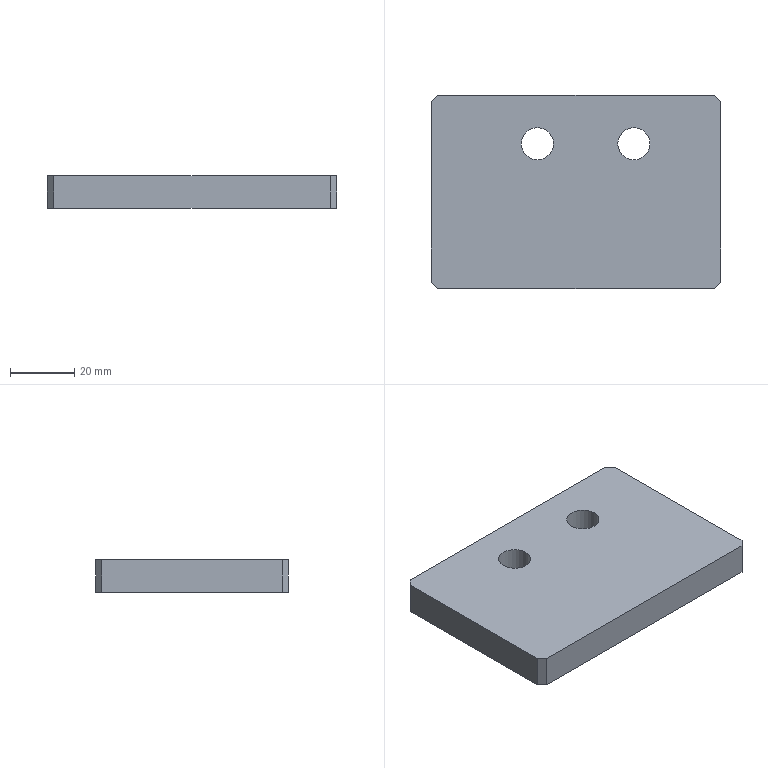NC program | NX | posted with a generic post | part box 90 x 60 x 10 mm
Lines 540 to 1827 of 1827:
(ADAPTIVE_MILLING_COPY , TOOL : D12开粗)
N1036 T02 M6
N1038 G54
N1040 G17 G0 G90 X-59.569 Y-30.89 S3000 M3
N1042 G43 Z20. H2
N1044 Z3.1
N1046 G94 G1 X-59.419 Y-30.888 Z2.163 F1500.
N1048 X-59.269 Y-30.885 Z1.792
N1050 X-59.119 Y-30.883 Z1.52
N1052 X-58.969 Y-30.88 Z1.3
N1054 X-58.819 Y-30.878 Z1.116
N1056 X-58.669 Y-30.875 Z0.958
N1058 X-58.519 Y-30.873 Z0.82
N1060 X-58.369 Y-30.87 Z0.7
N1062 X-58.219 Y-30.867 Z0.595
N1064 X-58.069 Y-30.865 Z0.502
N1066 X-57.919 Y-30.862 Z0.421
N1068 X-57.769 Y-30.86 Z0.35
N1070 X-57.619 Y-30.857 Z0.29
N1072 X-57.469 Y-30.855 Z0.238
N1074 X-57.319 Y-30.852 Z0.195
N1076 X-57.169 Y-30.85 Z0.161
N1078 X-57.019 Y-30.847 Z0.134
N1080 X-56.869 Y-30.845 Z0.115
N1082 X-56.719 Y-30.842 Z0.104
N1084 X-56.569 Y-30.84 Z0.1
N1086 X-54.659 Y-30.808
N1088 G3 X-53.548 Y-30.03 R1.212
N1090 X-53.17 Y-27.731 R8.892
N1092 X-53.004 Y-19.97 R127.75
N1094 G1 X-52.999 Y-14.169
N1096 X-52.997 Y32.519
N1098 G2 X-50.378 Y37.762 R6.759
N1100 X-45.571 Y39.899 R11.024
N1102 X-39.916 Y40.431 R33.002
N1104 X-28.979 Y40.499 R545.05
N1106 G1 X45.014 Y40.497
N1108 G2 X50.26 Y37.882 R6.758
N1110 X52.398 Y33.076 R11.015
N1112 X52.936 Y27.233 R33.716
N1114 X52.998 Y16.484 R602.889
N1116 G1 X52.997 Y-32.512
N1118 G2 X50.383 Y-37.757 R6.757
N1120 X45.576 Y-39.897 R11.021
N1122 X39.734 Y-40.436 R33.627
N1124 X28.984 Y-40.499 R598.92
N1126 G1 X-45.011 Y-40.497
N1128 G2 X-50.217 Y-37.931 R6.744
N1130 X-52.518 Y-31.955 R10.821
N1132 X-52.587 Y-26.958 R47.485
N1134 G3 X-52.499 Y-14.793 R707.62
N1136 G1 X-52.497 Y30.394
N1138 G2 X-48.711 Y37.306 R8.485
N1140 X-43.265 Y39.414 R13.689
N1142 X-36.542 Y39.944 R43.936
N1144 X-25.855 Y39.998 R696.998
N1146 G1 X42.893 Y39.997
N1148 G2 X49.808 Y36.209 R8.485
N1150 X51.913 Y30.767 R13.682
N1152 X52.446 Y23.92 R44.535
N1154 X52.498 Y12.92 R714.019
N1156 G1 X52.496 Y-30.39
N1158 G2 X48.799 Y-37.243 R8.475
N1160 X43.429 Y-39.382 R13.467
N1162 X37.022 Y-39.932 R40.74
N1164 X25.522 Y-39.998 R644.298
N1166 G1 X-42.89 Y-39.997
N1168 G2 X-50.102 Y-35.708 R8.457
N1170 X-51.749 Y-30.501 R13.432
N1172 X-52.014 Y-24.698 R49.366
N1174 G1 X-51.999 Y-15.168
N1176 X-51.998 Y28.27
N1178 G2 X-47.019 Y37.045 R9.749
N1180 X-41.174 Y38.973 R16.302
N1182 X-33.945 Y39.451 R55.428
N1184 X-24.32 Y39.498 R682.976
N1186 G1 X40.792 Y39.497
N1188 G2 X49.543 Y34.524 R9.746
N1190 X51.462 Y28.74 R16.226
N1192 X51.953 Y21.325 R55.538
N1194 X51.997 Y10.762 R717.555
N1196 G1 X51.996 Y-28.288
N1198 G2 X47.025 Y-37.04 R9.747
N1200 X41.178 Y-38.971 R16.292
N1202 X33.637 Y-39.456 R57.142
N1204 X23.324 Y-39.498 R714.456
N1206 G1 X-40.765 Y-39.497
N1208 G2 X-46.89 Y-37.527 R9.612
N1210 X-50.43 Y-32.205 R10.902
N1212 X-51.379 Y-26.298 R23.347
N1214 X-51.5 Y-18.487 R163.612
N1216 G1 X-51.498 Y26.444
N1218 G2 X-50.572 Y31.508 R12.25
N1220 X-45.244 Y36.861 R10.95
N1222 X-39.06 Y38.556 R19.433
N1224 X-31.012 Y38.967 R74.188
N1226 G1 X-21.199 Y38.997
N1228 X38.956 Y38.996
N1230 G2 X44.075 Y38.04 R12.18
N1232 X49.414 Y32.633 R10.992
N1234 X51.055 Y26.564 R19.568
N1236 X51.465 Y18.641 R73.264
N1238 G1 X51.497 Y8.829
N1240 X51.496 Y-26.453
N1242 G2 X50.54 Y-31.573 R12.182
N1244 X45.238 Y-36.861 R10.959
N1246 X39.116 Y-38.548 R19.361
N1248 X30.943 Y-38.967 R74.081
N1250 G1 X21.131 Y-38.998
N1252 X-38.953 Y-38.996
N1254 G2 X-43.781 Y-38.15 R12.071
N1256 X-49.101 Y-32.875 R10.495
N1258 X-50.645 Y-27.041 R18.389
N1260 X-50.984 Y-19.239 R74.744
N1262 G1 X-50.999 Y-11.614
N1264 X-50.998 Y24.811
N1266 G2 X-50.358 Y29.622 R15.163
N1268 X-44.803 Y36.031 R11.276
N1270 X-38.427 Y37.958 R19.18
N1272 X-30.26 Y38.454 R66.913
N1274 X-19.698 Y38.497 R723.605
N1276 G1 X37.331 Y38.496
N1278 G2 X42.141 Y37.851 R15.119
N1280 X48.569 Y32.23 R11.299
N1282 X50.442 Y26.038 R19.12
N1284 X50.948 Y18.06 R64.164
N1286 X50.997 Y6.748 R739.344
N1288 G1 X50.995 Y-24.828
N1290 G2 X50.331 Y-29.698 R15.054
N1292 X44.729 Y-36.069 R11.307
N1294 X38.472 Y-37.951 R19.238
N1296 X30.305 Y-38.453 R66.231
N1298 X19.993 Y-38.497 R712.26
N1300 G1 X-37.328 Y-38.496
N1302 G2 X-42.015 Y-37.872 R14.739
N1304 X-48.266 Y-32.372 R10.913
N1306 X-50.058 Y-26.153 R18.659
N1308 X-50.464 Y-18.856 R65.496
N1310 X-50.499 Y-8.919 R714.694
N1312 G1 Y22.955
N1314 G2 X-50.093 Y27.677 R20.632
N1316 X-44.089 Y35.381 R11.711
N1318 X-37.741 Y37.378 R19.475
N1320 X-29.766 Y37.935 R61.44
N1322 X-17.704 Y37.997 R739.177
N1324 G1 X35.581 Y37.996
N1326 G2 X40.359 Y37.548 R19.649
N1328 X47.878 Y31.593 R11.713
N1330 X49.877 Y25.245 R19.451
N1332 X50.432 Y17.396 R60.715
N1334 X50.496 Y4.959 R746.772
N1336 G1 Y-23.078
N1338 G2 X50.048 Y-27.857 R19.657
N1340 X44.094 Y-35.376 R11.714
N1342 X37.561 Y-37.405 R19.666
N1344 X29.334 Y-37.944 R65.096
N1346 X17.397 Y-37.997 R755.241
N1348 G1 X-35.716 Y-37.996
N1350 G2 X-40.426 Y-37.51 R18.131
N1352 X-47.589 Y-31.648 R11.386
N1354 X-49.483 Y-25.329 R19.143
N1356 X-49.957 Y-17.473 R65.04
N1358 X-49.999 Y-7.161 R715.418
N1360 G1 X-49.998 Y21.58
N1362 G2 X-49.606 Y26.555 R23.599
N1364 X-43.258 Y34.825 R12.177
N1366 X-36.784 Y36.851 R20.187
N1368 X-28.498 Y37.433 R63.335
N1370 X-16.498 Y37.496 R737.911
N1372 G1 X34.081
N1374 G2 X39.055 Y37.104 R23.631
N1376 X47.327 Y30.753 R12.176
N1378 X49.38 Y24.095 R20.39
N1380 X49.94 Y15.619 R66.815
N1382 X49.996 Y4.619 R715.925
N1384 G1 X49.995 Y-21.64
N1386 G2 X49.604 Y-26.553 R23.37
N1388 X43.254 Y-34.825 R12.176
N1390 X36.759 Y-36.854 R20.234
N1392 X28.598 Y-37.431 R62.902
N1394 X15.911 Y-37.497 R756.324
N1396 G1 X-33.953 Y-37.496
N1398 G2 X-38.744 Y-37.149 R24.037
N1400 X-46.94 Y-30.942 R11.836
N1402 X-48.929 Y-24.45 R19.689
N1404 X-49.45 Y-16.285 R65.25
N1406 X-49.498 Y-4.973 R739.456
N1408 G1 X-49.497 Y20.205
N1410 G2 X-49.14 Y25.372 R27.452
N1412 X-42.409 Y34.302 R12.608
N1414 X-35.615 Y36.366 R21.2
N1416 X-27.015 Y36.937 R68.595
N1418 X-14.64 Y36.996 R759.565
N1420 G1 X32.706 Y36.995
N1422 G2 X37.873 Y36.638 R27.447
N1424 X46.761 Y29.985 R12.59
N1426 X48.823 Y23.395 R20.784
N1428 X49.422 Y15.173 R63.113
N1430 X49.496 Y2.111 R755.001
N1432 G1 X49.495 Y-20.203
N1434 G2 X49.138 Y-25.37 R27.447
N1436 X42.431 Y-34.288 R12.598
N1438 X35.769 Y-36.341 R20.997
N1440 X27.358 Y-36.93 R65.469
N1442 X14.609 Y-36.996 R758.776
N1444 G1 X-32.64
N1446 G2 X-37.683 Y-36.651 R26.828
N1448 X-46.442 Y-30.007 R12.311
N1450 X-48.398 Y-23.508 R20.608
N1452 X-48.942 Y-15.282 R65.734
N1454 X-48.998 Y-3.282 R748.174
N1456 G1 X-48.997 Y18.956
N1458 G2 X-48.654 Y24.312 R30.683
N1460 X-41.645 Y33.754 R12.991
N1462 X-34.923 Y35.817 R21.6
N1464 X-26.388 Y36.424 R66.253
N1466 X-13.326 Y36.496 R760.292
N1468 G1 X31.456 Y36.495
N1470 G2 X36.813 Y36.152 R30.68
N1472 X46.257 Y29.139 R12.991
N1474 X48.327 Y22.351 R21.706
N1476 X48.928 Y13.69 R67.775
N1478 X48.995 Y1.003 R755.917
N1480 G1 X48.994 Y-19.016
N1482 G2 X48.652 Y-24.31 R30.377
N1484 X41.639 Y-33.755 R12.989
N1486 X34.852 Y-35.826 R21.702
N1488 X26.255 Y-36.427 R67.324
N1490 X13.192 Y-36.496 R761.577
N1492 G1 X-31.453 Y-36.495
N1494 G2 X-36.623 Y-36.161 R29.577
N1496 X-45.833 Y-29.326 R12.696
N1498 X-47.872 Y-22.599 R21.178
N1500 X-48.44 Y-14.061 R67.815
N1502 X-48.497 Y-2.061 R748.385
N1504 G1 X-48.496 Y17.768
N1506 G2 X-48.163 Y23.313 R33.923
N1508 X-40.875 Y33.225 R13.35
N1510 X-33.967 Y35.314 R22.312
N1512 X-25.306 Y35.923 R68.534
N1514 X-11.932 Y35.995 R770.057
N1516 G1 X30.368 Y35.994
N1518 G2 X35.913 Y35.644 R32.71
N1520 X45.724 Y28.375 R13.34
N1522 X47.814 Y21.465 R22.311
N1524 X48.421 Y12.868 R68.251
N1526 X48.495 Y0.868 R720.862
N1528 G1 X48.493 Y-17.869
N1530 G2 X48.143 Y-23.414 R32.688
N1532 X40.876 Y-33.222 R13.341
N1534 X34.028 Y-35.303 R22.252
N1536 X25.431 Y-35.92 R67.417
N1538 X11.994 Y-35.995 R766.793
N1540 G1 X-30.306 Y-35.994
N1542 G2 X-35.725 Y-35.649 R31.627
N1544 X-45.278 Y-28.579 R13.059
N1546 X-47.349 Y-21.726 R21.763
N1548 X-47.936 Y-13.002 R69.124
N1550 X-47.997 Y-0.628 R755.649
N1552 G1 X-47.995 Y16.768
N1554 G2 X-47.646 Y22.5 R35.2
N1556 X-40.091 Y32.716 R13.677
N1558 X-33.167 Y34.793 R22.909
N1560 X-24.32 Y35.42 R69.666
N1562 X-10.571 Y35.495 R775.803
N1564 G1 X29.081 Y35.494
N1566 G2 X34.816 Y35.174 R37.476
N1568 X45.214 Y27.595 R13.684
N1570 X47.292 Y20.671 R22.893
N1572 X47.917 Y11.949 R69.041
N1574 X47.994 Y-0.426 R727.241
N1576 G1 X47.993 Y-16.578
N1578 G2 X47.674 Y-22.313 R37.496
N1580 X40.088 Y-32.716 R13.688
N1582 X33.17 Y-34.791 R22.924
N1584 X24.449 Y-35.417 R68.877
N1586 X10.699 Y-35.495 R772.946
N1588 G1 X-29.015 Y-35.494
N1590 G2 X-34.563 Y-35.187 R36.616
N1592 X-44.84 Y-27.629 R13.457
N1594 X-46.857 Y-20.695 R22.84
N1596 X-47.434 Y-11.907 R72.379
N1598 X-47.497 Y0.717 R763.165
N1600 G1 X-47.495 Y15.518
N1602 G2 X-47.192 Y21.317 R40.767
N1604 X-43.007 Y29.661 R14.033
N1606 X-36.223 Y33.426 R16.757
N1608 X-28.467 Y34.699 R35.764
N1610 X-17.473 Y34.984 R174.966
N1612 G1 X-9.91 Y34.995
N1614 X27.893 Y34.994
N1616 G2 X33.817 Y34.69 R41.623
N1618 X42.07 Y30.6 R14.047
N1620 X45.925 Y23.728 R16.697
N1622 X47.203 Y15.909 R35.882
N1624 X47.483 Y5.102 R175.284
N1626 G1 X47.494 Y-3.148
N1628 X47.493 Y-15.391
N1630 G2 X47.19 Y-21.315 R41.672
N1632 X43.102 Y-29.567 R14.047
N1634 X36.466 Y-33.35 R16.55
N1636 X28.783 Y-34.675 R34.459
N1638 X17.602 Y-34.983 R165.961
N1640 G1 X9.352 Y-34.995
N1642 X-27.828 Y-34.994
N1644 G2 X-33.565 Y-34.7 R40.526
N1646 X-42.02 Y-30.309 R13.761
N1648 X-45.559 Y-23.6 R16.821
N1650 X-46.723 Y-16.14 R36.323
N1652 X-46.991 Y-4.082 R198.021
N1654 G1 X-46.996 Y2.105
N1656 X-46.995 Y14.33
N1658 G2 X-46.71 Y20.319 R45.501
N1660 X-43.484 Y27.928 R14.662
N1662 X-36.738 Y32.487 R15.777
N1664 X-29.233 Y34.056 R30.463
N1666 X-18.932 Y34.467 R120.399
N1668 G1 X-9.307 Y34.494
N1670 X26.831 Y34.493
N1672 G2 X32.819 Y34.208 R45.449
N1674 X40.428 Y30.98 R14.652
N1676 X44.955 Y24.323 R15.724
N1678 X46.547 Y16.82 R30.062
N1680 X46.967 Y6.456 R119.196
N1682 G1 X46.994 Y-3.168
N1684 G2 X46.958 Y-17.015 R894.236
N1686 X46.166 Y-22.883 R22.934
N1688 X38.883 Y-31.545 R14.131
N1690 X31.739 Y-33.737 R23.419
N1692 X22.77 Y-34.407 R69.21
N1694 X8.708 Y-34.494 R725.36
N1696 G1 X-26.703 Y-34.493
N1698 G2 X-32.752 Y-34.189 R42.972
N1700 X-40.769 Y-30.384 R14.184
N1702 X-44.818 Y-23.562 R16.298
N1704 X-46.175 Y-15.822 R34.003
N1706 X-46.484 Y-4.829 R161.702
N1708 G1 X-46.496 Y3.421
N1710 G2 X-46.454 Y16.267 R676.278
N1712 X-45.584 Y22.374 R22.998
N1714 X-38.26 Y30.986 R14.365
N1716 X-30.939 Y33.231 R23.843
N1718 X-21.72 Y33.909 R71.389
N1720 X-7.283 Y33.994 R768.457
N1722 G1 X25.643 Y33.993
N1724 G2 X32.007 Y33.702 R49.117
N1726 X39.552 Y30.628 R15.084
N1728 X44.364 Y23.794 R15.81
N1730 X46.022 Y16.18 R30.054
N1732 X46.463 Y5.818 R115.982
N1734 G1 X46.493 Y-3.807
N1736 G2 X46.451 Y-16.265 R648.348
N1738 X45.582 Y-22.372 R22.999
N1740 X38.265 Y-30.981 R14.361
N1742 X31.185 Y-33.19 R23.535
N1744 X22.095 Y-33.899 R67.862
N1746 X7.283 Y-33.994 R698.792
N1748 G1 X-25.578 Y-33.993
N1750 G2 X-31.754 Y-33.707 R47.373
N1752 X-39.296 Y-30.574 R14.789
N1754 X-43.946 Y-23.834 R15.682
N1756 X-45.535 Y-16.46 R29.732
N1758 X-45.967 Y-6.16 R115.012
N1760 G1 X-45.996 Y4.153
N1762 G2 X-45.941 Y15.704 R452.456
N1764 X-45.004 Y21.863 R22.721
N1766 X-37.557 Y30.474 R14.601
N1768 X-30.234 Y32.712 R24.223
N1770 X-21.016 Y33.402 R71.367
N1772 X-7.267 Y33.493 R695.731
N1774 G1 X24.518
N1776 G2 X31.008 Y33.224 R54.432
N1778 X38.224 Y30.603 R15.779
N1780 X43.579 Y23.756 R15.519
N1782 X45.418 Y16.253 R28.081
N1784 X45.942 Y6.459 R95.891
N1786 X45.993 Y-5.229 R761.677
N1788 X45.938 Y-15.702 R398.582
N1790 X45.002 Y-21.862 R22.729
N1792 X37.562 Y-30.469 R14.6
N1794 X30.239 Y-32.71 R24.23
N1796 X21.021 Y-33.402 R71.255
N1798 X7.272 Y-33.494 R689.902
N1800 G1 X-24.453 Y-33.493
N1802 G2 X-30.755 Y-33.227 R52.481
N1804 X-38.002 Y-30.53 R15.452
N1806 X-43.165 Y-23.783 R15.41
N1808 X-44.952 Y-16.331 R28.096
N1810 X-45.455 Y-6.223 R100.534
N1812 X-45.495 Y5.527 R787.676
N1814 X-45.422 Y15.263 R274.803
N1816 X-44.387 Y21.468 R22.131
N1818 X-36.847 Y29.973 R14.832
N1820 X-29.458 Y32.207 R24.724
N1822 X-20.615 Y32.889 R70.497
N1824 X-6.554 Y32.993 R617.429
N1826 G1 X23.496 Y32.992
N1828 G2 X30.175 Y32.725 R57.816
N1830 X37.319 Y30.25 R16.264
N1832 X42.997 Y23.22 R15.591
N1834 X44.889 Y15.664 R28.061
N1836 X45.436 Y5.872 R93.584
N1838 X45.452 Y-14.365 R851.165
N1840 X44.651 Y-20.61 R25.74
N1842 X36.94 Y-29.922 R14.805
N1844 X29.563 Y-32.188 R24.482
N1846 X20.347 Y-32.895 R70.992
N1848 X5.222 Y-32.993 R705.308
N1850 G1 X-23.328
N1852 G2 X-29.757 Y-32.747 R58.397
N1854 X-36.853 Y-30.339 R16.169
N1856 X-42.475 Y-23.489 R15.342
N1858 X-44.388 Y-16.004 R27.328
N1860 X-44.938 Y-6.337 R90.537
N1862 X-44.955 Y13.462 R849.616
N1864 X-44.195 Y19.714 R27.14
N1866 X-36.224 Y29.433 R15.024
N1868 X-28.84 Y31.68 R24.95
N1870 X-19.873 Y32.384 R70.359
N1872 X-5.124 Y32.493 R628.055
N1874 G1 X22.364 Y32.492
N1876 G2 X29.23 Y32.242 R63.749
N1878 X36.313 Y29.956 R16.939
N1880 X42.282 Y22.995 R15.551
N1882 X44.29 Y15.602 R26.857
N1884 X44.918 Y5.941 R83.161
N1886 X44.953 Y-13.434 R753.505
N1888 X44.216 Y-19.626 R27.436
N1890 X36.229 Y-29.428 R15.023
N1892 X28.905 Y-31.667 R24.864
N1894 X19.565 Y-32.392 R71.306
N1896 X5.565 Y-32.493 R648.052
N1898 G1 X-22.297 Y-32.492
N1900 G2 X-29.038 Y-32.235 R60.414
N1902 X-36.095 Y-29.882 R16.519
N1904 X-41.891 Y-22.954 R15.463
N1906 X-43.841 Y-15.54 R27.151
N1908 X-44.421 Y-6.313 R84.039
N1910 X-44.454 Y12.624 R716.587
N1912 X-43.689 Y19.001 R27.965
N1914 X-35.694 Y28.851 R15.184
N1916 X-28.318 Y31.139 R24.924
N1918 X-18.917 Y31.886 R70.795
N1920 X-4.168 Y31.992 R650.065
N1922 G1 X21.382
N1924 G2 X28.499 Y31.735 R66.483
N1926 X35.592 Y29.484 R17.303
N1928 X41.782 Y22.296 R15.734
N1930 X43.805 Y14.709 R27.55
N1932 X44.415 Y5.172 R85.471
N1934 X44.443 Y-12.89 R576.077
N1936 X43.634 Y-19.198 R26.829
N1938 X35.654 Y-28.869 R15.193
N1940 X28.395 Y-31.124 R24.881
N1942 X19.183 Y-31.878 R68.93
N1944 X4.372 Y-31.992 R603.076
N1946 G1 X-21.241
N1948 G2 X-28.108 Y-31.75 R66.124
N1950 X-35.101 Y-29.572 R17.199
N1952 X-41.277 Y-22.496 R15.514
N1954 X-43.316 Y-14.918 R27.092
N1956 X-43.917 Y-5.567 R83.745
N1958 X-43.941 Y12.182 R531.225
N1960 X-43.133 Y18.491 R27.342
N1962 X-34.96 Y28.379 R15.385
N1964 X-27.391 Y30.667 R25.652
N1966 X-18.113 Y31.384 R73.258
N1968 X-3.676 Y31.492 R634.739
N1970 G1 X20.436 Y31.491
N1972 G2 X27.554 Y31.253 R72.029
N1974 X34.58 Y29.182 R18.034
N1976 X41.11 Y21.983 R15.725
N1978 X43.255 Y14.301 R27.03
N1980 X43.899 Y5.017 R80.432
N1982 X43.939 Y-12.17 R476.093
N1984 X43.101 Y-18.6 R27.123
N1986 X35.048 Y-28.331 R15.368
N1988 X27.481 Y-30.65 R25.445
N1990 X18.142 Y-31.383 R72.387
N1992 X3.705 Y-31.492 R624.013
N1994 G1 X-20.283
N1996 G2 X-27.338 Y-31.247 R68.888
N1998 X-34.344 Y-29.119 R17.608
N2000 X-40.673 Y-22.025 R15.612
N2002 X-42.762 Y-14.52 R26.795
N2004 X-43.416 Y-4.736 R82.159
N2006 X-43.431 Y11.638 R423.949
N2008 X-42.52 Y18.183 R26.615
N2010 X-34.485 Y27.778 R15.517
N2012 X-26.992 Y30.11 R25.374
N2014 X-17.592 Y30.875 R70.853
N2016 X-1.718 Y30.992 R642.346
N2018 G1 X19.394 Y30.991
N2020 G2 X26.7 Y30.762 R77.721
N2022 X33.645 Y28.828 R18.692
N2024 X40.553 Y21.428 R15.817
N2026 X42.688 Y14.001 R26.751
N2028 X43.386 Y4.658 R76.209
N2030 X43.427 Y-11.653 R377.553
N2032 X42.548 Y-18.077 R26.764
N2034 X34.433 Y-27.802 R15.525
N2036 X26.811 Y-30.137 R25.703
N2038 X17.41 Y-30.88 R72.888
N2040 X2.598 Y-30.992 R628.724
N2042 G1 X-19.202 Y-30.991
N2044 G2 X-26.445 Y-30.76 R75.302
N2046 X-33.317 Y-28.816 R18.354
N2048 X-40.105 Y-21.484 R15.693
N2050 X-42.226 Y-13.994 R26.769
N2052 X-42.902 Y-4.461 R78.861
N2054 X-42.931 Y10.788 R372.385
N2056 X-42.079 Y17.279 R27.95
N2058 X-33.849 Y27.265 R15.69
N2060 X-26.231 Y29.615 R25.836
N2062 X-16.768 Y30.375 R72.478
N2064 X-0.644 Y30.491 R659.501
N2066 G1 X18.469
N2068 G2 X26.087 Y30.247 R78.624
N2070 X33.081 Y28.278 R18.867
N2072 X40.029 Y20.81 R15.986
N2074 X42.206 Y13.139 R27.259
N2076 X42.899 Y3.295 R81.438
N2078 X42.912 Y-11.203 R300.444
N2080 X41.943 Y-17.739 R25.936
N2082 X33.873 Y-27.25 R15.671
N2084 X26.315 Y-29.598 R25.708
N2086 X16.791 Y-30.374 R71.856
N2088 X0.605 Y-30.492 R657.571
N2090 G1 X-18.258 Y-30.491
N2092 G2 X-25.751 Y-30.252 R77.544
N2094 X-32.685 Y-28.299 R18.637
N2096 X-39.548 Y-20.929 R15.832
N2098 X-41.697 Y-13.441 R26.817
N2100 X-42.395 Y-3.91 R77.606
N2102 X-42.41 Y10.526 R282.113
N2104 X-41.425 Y17.122 R26.283
N2106 X-33.161 Y26.782 R15.842
N2108 X-25.472 Y29.121 R26.31
N2110 X-16.196 Y29.867 R72.956
N2112 X-0.759 Y29.991 R604.001
N2114 G1 X18.228 Y29.989
N2116 G2 X25.657 Y29.714 R71.025
N2118 X32.744 Y27.609 R18.72
N2120 X39.519 Y20.172 R16.182
N2122 X41.675 Y12.617 R27.376
N2124 X42.387 Y2.962 R78.943
N2126 X42.4 Y-10.662 R247.08
N2128 X41.364 Y-17.311 R25.587
N2130 X33.234 Y-26.742 R15.823
N2132 X25.551 Y-29.105 R26.114
N2134 X16.151 Y-29.868 R72.626
N2136 X-0.598 Y-29.991 R659.571
N2138 G1 X-18.086 Y-29.989
N2140 G2 X-25.265 Y-29.724 R69.895
N2142 X-32.352 Y-27.623 R18.514
N2144 X-39.025 Y-20.31 R16.022
N2146 X-41.216 Y-12.573 R27.344
N2148 X-41.897 Y-2.978 R80.637
N2150 X-41.907 Y9.77 R242.832
N2152 X-40.912 Y16.49 R26.77
N2154 X-32.66 Y26.208 R15.965
N2156 X-24.853 Y28.605 R26.385
N2158 X-15.453 Y29.366 R73.385
N2160 X-0.079 Y29.49 R599.195
N2162 G1 X17.284 Y29.489
N2164 G2 X24.714 Y29.237 R77.294
N2166 X31.725 Y27.309 R19.514
N2168 X38.898 Y19.773 R16.197
N2170 X41.172 Y11.925 R27.418
N2172 X41.881 Y2.394 R79.068
N2174 X41.897 Y-9.916 R214.326
N2176 X40.884 Y-16.571 R26.237
N2178 X32.666 Y-26.201 R15.961
N2180 X25.05 Y-28.57 R26.149
N2182 X15.59 Y-29.361 R71.472
N2184 X-1.221 Y-29.491 R631.424
N2186 G1 X-17.084 Y-29.489
N2188 G2 X-24.451 Y-29.233 R74.928
N2190 X-31.448 Y-27.261 R19.132
N2192 X-38.444 Y-19.822 R16.086
N2194 X-40.677 Y-12.102 R27.22
N2196 X-41.396 Y-2.197 R80.139
N2198 X-41.377 Y9.614 R184.313
N2200 X-40.256 Y16.312 R25.227
N2202 X-32.19 Y25.62 R16.061
N2204 X-24.345 Y28.073 R26.293
N2206 X-14.822 Y28.861 R72.746
N2208 X1.052 Y28.99 R601.271
N2210 G1 X16.415 Y28.989
N2212 G2 X24.094 Y28.726 R78.463
N2214 X31.163 Y26.769 R19.682
N2216 X38.339 Y19.252 R16.301
N2218 X40.612 Y11.603 R27.131
N2220 X41.364 Y2.202 R74.823
N2222 X41.369 Y-9.671 R170.277
N2224 X40.215 Y-16.426 R24.907
N2226 X32.048 Y-25.689 R16.091
N2228 X24.253 Y-28.086 R26.596
N2230 X14.729 Y-28.863 R73.64
N2232 X-1.77 Y-28.99 R633.569
N2234 G1 X-16.195 Y-28.989
N2236 G2 X-23.688 Y-28.736 R78.263
N2238 X-30.76 Y-26.785 R19.547
N2240 X-37.895 Y-19.273 R16.203
N2242 X-40.123 Y-11.734 R27.06
N2244 X-40.881 Y-1.958 R76.323
N2246 X-40.858 Y9.165 R153.521
N2248 X-39.648 Y15.974 R24.611
N2250 X-31.55 Y25.123 R16.195
N2252 X-23.88 Y27.535 R26.387
N2254 X-14.485 Y28.347 R70.631
N2256 X3.076 Y28.49 R612.418
N2258 G1 X15.564 Y28.488
N2260 G2 X23.369 Y28.227 R81.493
N2262 X30.451 Y26.31 R20.127
N2264 X37.811 Y18.672 R16.41
N2266 X40.122 Y10.842 R27.499
N2268 X40.867 Y1.315 R77.049
N2270 X40.844 Y-9.307 R137.405
N2272 X39.576 Y-16.166 R24.043
N2274 X31.564 Y-25.113 R16.188
N2276 X23.897 Y-27.53 R26.352
N2278 X14.19 Y-28.356 R71.737
N2280 X-3.059 Y-28.49 R637.467
N2282 G1 X-15.359 Y-28.489
N2284 G2 X-23.164 Y-28.216 R77.999
N2286 X-30.168 Y-26.261 R19.64
N2288 X-37.355 Y-18.711 R16.321
N2290 X-39.617 Y-11.067 R27.252
N2292 X-40.372 Y-1.478 R75.896
N2294 X-40.338 Y8.707 R128.277
N2296 X-39.084 Y15.506 R24.307
N2298 X-30.834 Y24.667 R16.35
N2300 X-23.096 Y27.052 R26.895
N2302 X-13.512 Y27.854 R73.287
N2304 X2.299 Y27.989 R579.941
N2306 G1 X13.974
N2308 G2 X22.157 Y27.775 R101.775
N2310 X29.121 Y26.14 R21.677
N2312 X37.237 Y18.192 R16.437
N2314 X39.567 Y10.501 R27.207
N2316 X40.358 Y0.852 R74.548
N2318 X40.298 Y-9.206 R109.209
N2320 X38.835 Y-16.149 R22.673
N2322 X30.749 Y-24.707 R16.385
N2324 X22.94 Y-27.075 R27.229
N2326 X13.292 Y-27.86 R75.193
N2328 X-3.582 Y-27.99 R647.562
N2330 X-18.757 Y-27.94 R864.103
N2332 X-25.64 Y-27.181 R33.424
N2334 X-36.725 Y-18.34 R16.299
N2336 X-39.082 Y-10.589 R26.983
N2338 X-39.862 Y-1.003 R74.177
N2340 X-39.799 Y8.494 R104.034
N2342 X-38.389 Y15.386 R23.175
N2344 X-30.355 Y24.094 R16.44
N2346 X-22.504 Y26.537 R26.921
N2348 X-12.67 Y27.357 R74.351
N2350 X4.204 Y27.489 R637.079
N2352 X18.566 Y27.432 R696.859
N2354 X25.386 Y26.67 R33.837
N2356 X36.665 Y17.712 R16.53
N2358 X39.043 Y9.968 R27.179
N2360 X39.852 Y0.259 R73.698
N2362 X39.754 Y-8.986 R88.643
N2364 X38.147 Y-15.961 R21.814
N2366 X30.213 Y-24.162 R16.498
N2368 X22.53 Y-26.531 R27.116
N2370 X12.947 Y-27.348 R72.791
N2372 X-4.302 Y-27.489 R612.109
N2374 X-18.164 Y-27.436 R705.169
N2376 X-24.925 Y-26.694 R33.811
N2378 X-36.15 Y-17.858 R16.408
N2380 X-38.566 Y-10. R27.009
N2382 X-39.362 Y-0.165 R74.573
N2384 X-39.212 Y8.766 R78.147
N2386 X-37.433 Y15.821 R21.127
N2388 X-29.722 Y23.601 R16.62
N2390 X-21.804 Y26.042 R27.289
N2392 X-11.97 Y26.855 R75.298
N2394 X5.591 Y26.989 R665.399
N2396 X18.141 Y26.922 R475.392
N2398 X25.016 Y26.101 R32.712
N2400 X36.103 Y17.217 R16.616
N2402 X38.532 Y9.36 R27.251
N2404 X39.358 Y-0.849 R74.986
N2406 X39.151 Y-9.278 R65.815
N2408 X37.028 Y-16.617 R19.872
N2410 X29.337 Y-23.788 R16.798
N2412 X21.385 Y-26.107 R28.319
N2414 X11.545 Y-26.867 R79.925
N2416 X-5.641 Y-26.989 R710.751
N2418 X-17.941 Y-26.919 R462.341
N2420 X-24.75 Y-26.076 R31.722
N2422 X-35.662 Y-17.211 R16.52
N2424 X-38.062 Y-9.343 R27.327
N2426 X-38.867 Y1.055 R75.86
N2428 X-38.6 Y9.044 R58.071
N2430 X-36.222 Y16.561 R19.338
N2432 X-28.623 Y23.337 R17.032
N2434 X-20.717 Y25.61 R28.757
N2436 X-10.565 Y26.374 R82.211
N2438 X6.185 Y26.488 R740.157
N2440 X17.921 Y26.403 R365.762
N2442 X24.905 Y25.462 R30.659
N2444 X35.617 Y16.575 R16.714
N2446 X38.019 Y8.775 R27.456
N2448 X38.855 Y-1.934 R74.521
N2450 X38.508 Y-9.668 R49.416
N2452 X35.646 Y-17.467 R18.35
N2454 X28.058 Y-23.591 R17.411
N2456 X19.917 Y-25.724 R30.66
N2458 X9.882 Y-26.391 R91.673
N2460 X-6.18 Y-26.489 R827.798
N2462 X-17.604 Y-26.404 R342.957
N2464 X-24.464 Y-25.48 R30.352
N2466 X-35.101 Y-16.715 R16.6
N2468 X-37.531 Y-8.859 R27.27
N2470 X-38.356 Y2.162 R73.988
N2472 X-37.899 Y9.701 R43.079
N2474 X-34.363 Y17.939 R17.684
N2476 X-26.789 Y23.366 R18.106
N2478 X-18.538 Y25.317 R33.062
N2480 X-7.685 Y25.92 R107.817
N2482 X16.177 Y25.937 R979.786
N2484 X23.132 Y25.241 R37.672
N2486 X32.415 Y19.992 R16.931
N2488 X36.536 Y12.375 R20.185
N2490 X38.057 Y3.647 R41.409
N2492 X38.184 Y-7.341 R71.9
N2494 X36.472 Y-14.479 R21.575
N2496 X28.595 Y-22.548 R16.767
N2498 X20.867 Y-24.975 R27.293
N2500 X11.1 Y-25.836 R72.257
N2502 X-4.773 Y-25.988 R534.9
N2504 X-16.573 Y-25.916 R422.533
N2506 X-23.446 Y-25.079 R32.747
N2508 X-34.615 Y-16.073 R16.735
N2510 X-37.049 Y-8.09 R27.715
N2512 X-37.69 Y6.556 R69.699
N2514 X-36.02 Y13.767 R22.033
N2516 X-27.886 Y22.104 R16.898
N2518 X-20.085 Y24.5 R27.822
N2520 X-10.253 Y25.341 R74.669
N2522 X7.996 Y25.488 R641.905
N2524 X17.618 Y25.35 R187.144
N2526 X24.623 Y24.167 R27.166
N2528 X34.52 Y15.553 R16.868
N2530 X36.978 Y7.708 R27.486
N2532 X37.658 Y-6.745 R64.982
N2534 X35.882 Y-14.056 R21.442
N2536 X28.049 Y-22.018 R16.848
N2538 X20.076 Y-24.499 R27.653
N2540 X10.182 Y-25.343 R74.979
N2542 X-8.379 Y-25.488 R662.9
N2544 X-17.813 Y-25.316 R149.817
N2546 X-24.844 Y-23.951 R24.906
N2548 X-34.01 Y-15.672 R16.758
N2550 X-36.471 Y-7.891 R27.18
N2552 X-37.134 Y6.313 R61.636
N2554 X-35.256 Y13.724 R21.174
N2556 X-27.379 Y21.555 R16.993
N2558 X-19.402 Y24.006 R28.009
N2560 X-9.319 Y24.848 R76.801
N2562 X10.242 Y24.985 R720.423
N2564 X18.548 Y24.731 R96.357
N2566 X25.691 Y23.022 R22.637
N2568 X34.057 Y14.879 R17.019
N2570 X36.486 Y7.016 R27.881
N2572 X37.098 Y-6.501 R57.979
N2574 X35.164 Y-13.896 R20.716
N2576 X27.4 Y-21.541 R16.98
N2578 X19.544 Y-23.979 R27.809
N2580 X9.651 Y-24.837 R74.318
N2582 X-7.973 Y-24.987 R606.953
N2584 X-17.344 Y-24.801 R140.292
N2586 X-24.485 Y-23.355 R24.579
N2588 X-33.522 Y-15.044 R16.877
N2590 X-35.999 Y-7.072 R27.632
N2592 X-36.571 Y6.072 R55.081
N2594 X-34.501 Y13.622 R20.438
N2596 X-26.673 Y21.108 R17.13
N2598 X-18.738 Y23.51 R28.397
N2600 X-8.843 Y24.341 R76.744
N2602 X14.343 Y24.429 R624.205
N2604 X21.481 Y23.687 R37.931
N2606 X30.89 Y18.284 R17.198
N2608 X35.002 Y10.621 R20.577
N2610 X36.534 Y1.707 R41.108
N2612 X36.436 Y-7.091 R45.003
N2614 X33.662 Y-15.048 R18.713
N2616 X26.057 Y-21.395 R17.566
N2618 X18.003 Y-23.623 R30.181
N2620 X7.599 Y-24.376 R87.43
N2622 X-13.963 Y-24.43 R650.97
N2624 X-21.039 Y-23.7 R37.771
N2626 X-30.411 Y-18.33 R17.121
N2628 X-34.524 Y-10.66 R20.478
N2630 X-36.067 Y-1.307 R41.38
N2632 X-35.828 Y7.174 R40.2
N2634 X-32.368 Y15.585 R17.989
N2636 X-24.868 Y21.155 R18.2
N2638 X-16.586 Y23.234 R32.378
N2640 X-6.174 Y23.893 R98.607
N2642 X13.7 Y23.927 R607.887
N2644 X20.839 Y23.192 R38.443
N2646 X30.102 Y18.032 R17.352
N2648 X34.413 Y10.297 R20.324
N2650 X36.02 Y1.019 R39.955
N2652 X35.772 Y-7.397 R37.879
N2654 X32.05 Y-15.971 R17.665
N2656 X24.477 Y-21.31 R18.497
N2658 X16.107 Y-23.292 R33.809
N2660 X5.567 Y-23.906 R106.059
N2662 X-13.432 Y-23.925 R582.633
N2664 X-20.568 Y-23.165 R37.31
N2666 X-30.148 Y-17.478 R17.155
N2668 X-34.125 Y-9.7 R21.032
N2670 X-35.597 Y0.67 R42.483
N2672 X-34.95 Y8.372 R30.167
N2674 X-26.018 Y19.836 R17.011
N2676 X-18.072 Y22.407 R27.456
N2678 X-8.059 Y23.32 R72.46
N2680 X13.626 Y23.408 R461.828
N2682 X20.812 Y22.554 R35.193
N2684 X32.461 Y13.289 R17.284
N2686 X34.976 Y5.124 R28.068
N2688 X35.395 Y-5.588 R41.825
N2690 X32.843 Y-13.56 R18.994
N2692 X25.245 Y-20.216 R17.484
N2694 X17.222 Y-22.547 R29.471
N2696 X7.073 Y-23.352 R81.593
N2698 X-12.988 Y-23.418 R484.689
N2700 X-20.18 Y-22.611 R36.336
N2702 X-32.012 Y-13.272 R17.231
N2704 X-34.475 Y-5.235 R27.91
N2706 X-34.837 Y5.352 R39.507
N2708 X-32.01 Y13.506 R18.587
N2710 X-24.283 Y19.891 R17.806
N2712 X-16.103 Y22.124 R30.836
N2714 X-5.448 Y22.878 R90.644
N2716 X13.05 Y22.904 R426.045
N2718 X20.236 Y22.047 R35.395
N2720 X31.978 Y12.668 R17.378
N2722 X34.496 Y4.32 R28.261
N2724 X34.752 Y-5.77 R36.667
N2726 X31.494 Y-14.225 R17.973
N2728 X24.045 Y-19.991 R18.035
N2730 X15.851 Y-22.158 R31.554
N2732 X5.444 Y-22.877 R92.417
N2734 X-12.43 Y-22.913 R435.621
N2736 X-19.622 Y-22.098 R36.317
N2738 X-31.57 Y-12.563 R17.344
N2740 X-34.038 Y-4.128 R28.447
N2742 X-34.194 Y5.465 R34.577
N2744 X-30.579 Y14.196 R17.711
N2746 X-22.934 Y19.713 R18.519
N2748 X-14.697 Y21.731 R33.384
N2750 X-3.723 Y22.4 R103.582
N2752 X12.464 Y22.4 R378.497
N2754 X19.589 Y21.556 R35.656
N2756 X31.514 Y12.01 R17.473
N2758 X34.043 Y3.279 R28.546
N2760 X34.088 Y-5.939 R31.995
N2762 X29.382 Y-15.523 R17.153
N2764 X21.714 Y-20.164 R19.709
N2766 X13.031 Y-21.92 R38.459
N2768 X1.546 Y-22.436 R135.714
N2770 X-12.328 Y-22.392 R331.645
N2772 X-19.566 Y-21.459 R33.675
N2774 X-30.976 Y-12.165 R17.36
N2776 X-33.527 Y-3.441 R27.999
N2778 X-33.497 Y5.773 R30.301
N2780 X-24.413 Y18.251 R17.04
N2782 X-16.544 Y20.846 R27.378
N2784 X-6.786 Y21.793 R69.619
N2786 X11.899 Y21.896 R331.385
N2788 X19.206 Y21.002 R35.211
N2790 X31.006 Y11.444 R17.536
N2792 X33.558 Y2.327 R28.289
N2794 X33.369 Y-6.262 R27.957
N2796 X24.584 Y-18.152 R16.907
N2798 X16.612 Y-20.829 R27.081
N2800 X6.668 Y-21.796 R69.521
N2802 X-11.642 Y-21.892 R315.771
N2804 X-18.943 Y-20.964 R34.19
N2806 X-30.512 Y-11.506 R17.449
N2808 X-33.068 Y-2.206 R27.923
N2810 X-32.686 Y6.433 R26.018
N2812 X-24.095 Y17.607 R16.893
N2814 X-16.247 Y20.286 R26.86
N2816 X-6.431 Y21.28 R67.377
N2818 X11.753 Y21.374 R279.376
N2820 X18.986 Y20.403 R33.25
N2822 X30.417 Y11.041 R17.547
N2824 X33.057 Y1.26 R27.57
N2826 X32.476 Y-7.113 R23.923
N2828 X24.326 Y-17.47 R16.757
N2830 X16.499 Y-20.232 R26.283
N2832 X6.688 Y-21.268 R65.183
N2834 X-11.183 Y-21.382 R276.75
N2836 X-18.361 Y-20.459 R34.003
N2838 X-29.975 Y-10.994 R17.504
N2840 X-32.588 Y-0.567 R27.33
N2842 X-31.582 Y7.757 R21.718
N2844 X-23.591 Y17.062 R16.836
N2846 X-15.688 Y19.776 R26.84
N2848 X-5.997 Y20.771 R66.856
N2850 X11.125 Y20.872 R253.335
N2852 X18.419 Y19.895 R33.512
N2854 X29.961 Y10.37 R17.619
N2856 X32.325 Y-4.49 R26.643
N2858 X23.602 Y-17.046 R16.76
N2860 X15.7 Y-19.77 R26.753
N2862 X6.073 Y-20.766 R66.434
N2864 X-10.923 Y-20.864 R239.349
N2866 X-18.15 Y-19.856 R32.433
N2868 X-29.467 Y-10.423 R17.536
N2870 X-31.766 Y4.07 R25.733
N2872 X-23.193 Y16.458 R16.734
N2874 X-15.128 Y19.266 R26.655
N2876 X-5.438 Y20.267 R66.806
N2878 X10.808 Y20.356 R221.483
N2880 X18.214 Y19.288 R32.19
N2882 X29.451 Y9.807 R17.642
N2884 X31.687 Y-4.193 R24.789
N2886 X23.448 Y-16.299 R16.563
N2888 X15.547 Y-19.178 R25.84
N2890 X5.991 Y-20.24 R62.727
N2892 X-10.38 Y-20.357 R214.434
N2894 X-17.605 Y-19.342 R32.417
N2896 X-29.004 Y-9.758 R17.593
N2898 X-31.124 Y3.768 R23.974
N2900 X-23.027 Y15.714 R16.517
N2902 X-15.203 Y18.628 R25.55
N2904 X-5.526 Y19.733 R61.559
N2906 X10.344 Y19.845 R196.966
N2908 X17.567 Y18.806 R32.215
N2910 X29.027 Y9.06 R17.703
N2912 X31.032 Y-3.92 R23.077
N2914 X23.052 Y-15.684 R16.374
N2916 X15.112 Y-18.642 R25.494
N2918 X5.684 Y-19.724 R61.211
N2920 X-9.936 Y-19.845 R190.455
N2922 X-17.218 Y-18.784 R31.771
N2924 X-28.524 Y-9.119 R17.604
N2926 X-30.462 Y3.491 R22.307
N2928 X-22.482 Y15.187 R16.341
N2930 X-14.611 Y18.125 R25.506
N2932 X-5.184 Y19.218 R60.86
N2934 X10.186 Y19.317 R170.224
N2936 X17.452 Y18.168 R30.478
N2938 X28.562 Y8.388 R17.703
N2940 X30.374 Y-3.567 R21.511
N2942 X22.736 Y-15.016 R16.147
N2944 X14.904 Y-18.057 R24.84
N2946 X5.483 Y-19.201 R58.516
N2948 X-9.698 Y-19.321 R166.023
N2950 X-17.027 Y-18.167 R30.321
N2952 X-28.13 Y-8.28 R17.612
N2954 X-29.777 Y3.263 R20.741
N2956 X-22.221 Y14.485 R16.087
N2958 X-14.396 Y17.541 R24.815
N2960 X-5.04 Y18.692 R58.104
N2962 X9.829 Y18.798 R151.279
N2964 X17.147 Y17.581 R29.581
N2966 X28.152 Y7.568 R17.675
N2968 X29.644 Y-3.553 R19.903
N2970 X22.401 Y-14.351 R15.89
N2972 X14.714 Y-17.462 R24.195
N2974 X5.429 Y-18.668 R55.463
N2976 X-9.315 Y-18.803 R147.939
N2978 X-16.576 Y-17.626 R29.809
N2980 X-27.78 Y-7.293 R17.591
N2982 X-28.993 Y3.492 R19.089
N2984 X-21.837 Y13.85 R15.83
N2986 X-13.976 Y16.999 R24.391
N2988 X-4.749 Y18.172 R56.517
N2990 X9.307 Y18.287 R137.168
N2992 X16.624 Y17.064 R29.496
N2994 X27.875 Y6.369 R17.643
N2996 X28.797 Y-4.006 R18.224
N2998 X21.948 Y-13.754 R15.66
N3000 X14.352 Y-16.905 R23.803
N3002 X5.134 Y-18.148 R53.913
N3004 X-8.922 Y-18.284 R132.213
N3006 X-16.235 Y-17.049 R29.137
N3008 X-27.539 Y-5.913 R17.531
N3010 X-27.977 Y4.477 R17.326
N3012 X-21.305 Y13.304 R15.662
N3014 X-13.636 Y16.438 R24.014
N3016 X-4.415 Y17.655 R54.838
N3018 X9.078 Y17.756 R120.834
N3020 X16.437 Y16.434 R28.254
N3022 X27.803 Y4.297 R17.538
N3024 X27.392 Y-5.953 R16.206
N3026 X20.702 Y-13.658 R15.832
N3028 X12.831 Y-16.612 R25.244
N3030 X3.092 Y-17.725 R61.718
N3032 X-8.778 Y-17.747 R113.145
N3034 X-16.189 Y-16.368 R27.499
N3036 X-27.707 Y1.942 R17.322
N3038 X-21.291 Y12.398 R15.134
N3040 X-13.727 Y15.766 R22.746
N3042 X-4.587 Y17.103 R50.448
N3044 X8.654 Y17.236 R109.308
N3046 X16.067 Y15.864 R27.745
N3048 X27.639 Y-1.335 R17.055
N3050 X21.549 Y-12.174 R14.845
N3052 X13.952 Y-15.697 R22.144
N3054 X4.883 Y-17.08 R48.815
N3056 X-8.482 Y-17.217 R103.537
N3058 X-15.996 Y-15.727 R26.536
N3060 X-27.061 Y-0.13 R16.771
N3062 X-21.303 Y11.425 R14.621
N3064 X-13.952 Y15.038 R21.409
N3066 X-5.276 Y16.503 R44.904
N3068 X8.586 Y16.689 R96.594
N3070 X16.029 Y15.166 R26.213
N3072 X26.794 Y1.698 R16.651
N3074 X21.433 Y-11.272 R14.347
N3076 X14.176 Y-14.96 R20.891
N3078 X5.322 Y-16.496 R43.906
N3080 X-8.103 Y-16.69 R93.779
N3082 X-15.607 Y-15.156 R26.037
N3084 X-25.881 Y-3.613 R16.447
N3086 X-21.042 Y10.618 R14.145
N3088 X-13.757 Y14.413 R20.577
N3090 X-4.848 Y15.985 R43.187
N3092 X8.139 Y16.166 R87.61
N3094 X15.635 Y14.597 R25.787
N3096 X25.317 Y4.689 R16.36
N3098 X21.204 Y-10.419 R13.865
N3100 X13.987 Y-14.327 R20.017
N3102 X5.4 Y-15.932 R41.176
N3104 X-7.835 Y-16.152 R84.035
N3106 X-15.322 Y-14.541 R25.237
N3108 X-24.473 Y-5.507 R16.113
N3110 X-20.969 Y9.603 R13.614
N3112 X-13.802 Y13.699 R19.417
N3114 X-5.298 Y15.384 R39.193
N3116 X7.747 Y15.636 R79.68
N3118 X15.352 Y13.981 R25.168
N3120 X23.993 Y5.883 R16.002
N3122 X20.94 Y-9.549 R13.333
N3124 X14.054 Y-13.594 R18.966
N3126 X5.628 Y-15.346 R37.687
N3128 X-7.602 Y-15.608 R75.468
N3130 X-15.124 Y-13.885 R24.308
N3132 X-23.234 Y-6.345 R15.715
N3134 X-20.631 Y8.771 R13.066
N3136 X-13.641 Y13.036 R18.566
N3138 X-5.162 Y14.832 R36.975
N3140 X7.507 Y15.091 R71.611
N3142 X14.976 Y13.397 R24.408
N3144 X22.787 Y6.497 R15.619
N3146 X20.596 Y-8.703 R12.782
N3148 X13.896 Y-12.919 R18.086
N3150 X5.559 Y-14.782 R35.365
N3152 X-7.418 Y-15.054 R67.648
N3154 X-14.971 Y-13.197 R23.32
N3156 X-22.279 Y-6.422 R15.142
N3158 X-20.293 Y7.881 R12.497
N3160 X-13.658 Y12.285 R17.529
N3162 X-5.468 Y14.222 R33.69
N3164 X7.382 Y14.531 R64.135
N3166 X14.874 Y12.689 R23.282
N3168 X21.968 Y6.272 R14.951
N3170 X20.326 Y-7.708 R12.199
N3172 X13.76 Y-12.215 R17.075
N3174 X5.645 Y-14.192 R32.763
N3176 X-7.016 Y-14.516 R61.489
N3178 X-14.499 Y-12.646 R22.818
N3180 X-21.224 Y-6.607 R14.609
N3182 X-19.953 Y6.914 R11.933
N3184 X-13.614 Y11.528 R16.489
N3186 X-5.653 Y13.611 R30.872
N3188 X7.19 Y13.97 R57.658
N3190 X14.653 Y12.019 R22.292
N3192 X21.108 Y6.062 R14.197
N3194 X19.902 Y-6.797 R11.643
N3196 X13.564 Y-11.511 R16.161
N3198 X5.546 Y-13.616 R30.549
N3200 X-6.861 Y-13.949 R55.197
N3202 X-14.252 Y-11.981 R21.768
N3204 X-20.434 Y-6.233 R13.767
N3206 X-19.31 Y6.235 R11.403
N3208 X-13.154 Y10.926 R15.84
N3210 X-5.4 Y13.05 R29.361
N3212 X7.127 Y13.389 R51.594
N3214 X14.542 Y11.276 R21.037
N3216 X20.364 Y5.551 R13.217
N3218 X19.215 Y-6.139 R11.134
N3220 X13.123 Y-10.892 R15.466
N3222 X5.437 Y-13.033 R28.715
N3224 X-6.653 Y-13.381 R49.605
N3226 X-13.955 Y-11.325 R20.756
N3228 X-19.649 Y-5.759 R12.803
N3230 X-18.73 Y5.391 R10.884
N3232 X-12.84 Y10.236 R14.973
N3234 X-5.182 Y12.477 R27.408
N3236 X6.904 Y12.817 R46.468
N3238 X14.002 Y10.737 R20.145
N3240 X19.418 Y5.34 R12.368
N3242 X18.52 Y-5.412 R10.64
N3244 X12.799 Y-10.195 R14.66
N3246 X5.15 Y-12.467 R26.816
N3248 X-6.624 Y-12.784 R44.232
N3250 X-13.696 Y-10.627 R19.382
N3252 X-18.878 Y-5.109 R11.746
N3254 X-17.804 Y4.957 R10.448
N3256 X-12.025 Y9.764 R14.519
N3258 X-4.557 Y11.96 R26.52
N3260 X6.78 Y12.226 R41.537
N3262 X13.711 Y10.043 R18.746
N3264 X18.706 Y4.465 R11.224
N3266 X17.471 Y-5.119 R10.251
N3268 X11.879 Y-9.765 R14.283
N3270 X4.47 Y-11.955 R26.058
N3272 X-6.554 Y-12.18 R39.335
N3274 X-13.174 Y-10.047 R18.013
N3276 X-18.031 Y-4.41 R10.749
N3278 X-16.739 Y4.649 R10.073
N3280 X-11.001 Y9.375 R14.171
N3282 X-3.446 Y11.508 R26.257
N3284 X6.894 Y11.588 R36.47
N3286 X13.239 Y9.418 R17.066
N3288 X17.941 Y3.273 R10.185
N3290 X16.149 Y-5.131 R10.009
N3292 X10.594 Y-9.488 R14.197
N3294 X2.897 Y-11.56 R26.468
N3296 X-6.881 Y-11.497 R33.747
N3298 X-12.988 Y-9.215 R15.694
N3300 X-17.39 Y-1.541 R9.554
N3302 X-14.435 Y5.811 R10.328
N3304 X-8.392 Y9.624 R15.57
N3306 X0.674 Y11.292 R30.66
N3308 X8.611 Y10.571 R26.645
N3310 X14.088 Y7.688 R12.69
N3312 X15.892 Y-3.378 R9.18
N3314 X10.836 Y-8.415 R12.497
N3316 X3.633 Y-10.815 R22.104
N3318 X-6.385 Y-10.931 R30.875
N3320 X-11.976 Y-8.862 R14.479
N3322 X-15.095 Y2.882 R8.984
N3324 X-10.093 Y7.933 R12.245
N3326 X-3.006 Y10.295 R21.477
N3328 X6.759 Y10.308 R28.485
N3330 X12.093 Y8.122 R13.051
N3332 X14.784 Y-2.796 R8.73
N3334 X10.041 Y-7.819 R11.809
N3336 X3.045 Y-10.246 R20.367
N3338 X-6.343 Y-10.265 R26.758
N3340 X-11.473 Y-8.08 R12.051
N3342 X-14.026 Y2.097 R8.488
N3344 X-9.402 Y7.248 R11.395
N3346 X-2.552 Y9.691 R19.355
N3348 X6.46 Y9.674 R24.722
N3350 X11.403 Y7.397 R10.944
N3352 X13.603 Y-2.111 R8.262
N3354 X9.099 Y-7.247 R11.081
N3356 X2.191 Y-9.695 R18.684
N3358 X-6.013 Y-9.619 R22.66
N3360 X-10.888 Y-7.166 R9.874
N3362 X-12.668 Y1.669 R8.06
N3364 X-8.164 Y6.825 R10.843
N3366 X-1.104 Y9.212 R18.205
N3368 X6.165 Y8.992 R20.013
N3370 X11.088 Y5.995 R8.728
N3372 X11.974 Y-2.167 R7.939
N3374 X7.379 Y-7.073 R10.816
N3376 X0.063 Y-9.258 R18.041
N3378 X-5.891 Y-8.85 R16.599
N3380 X-11.12 Y-4.301 R7.73
N3382 X-10.361 Y2.893 R8.086
N3384 X-5.217 Y7.228 R11.41
N3386 X4.688 Y8.5 R17.569
N3388 X9.777 Y5.286 R7.654
N3390 X10.182 Y-2.175 R7.594
N3392 X5.462 Y-6.882 R10.427
N3394 X-3.699 Y-8.456 R15.569
N3396 X-9.273 Y-4.155 R7.037
N3398 X-8.445 Y2.836 R7.683
N3400 X-3.206 Y6.936 R10.83
N3402 X3.167 Y7.824 R13.181
N3404 X8.843 Y0.298 R6.598
N3406 X5.368 Y-5.374 R8.573
N3408 X-1.594 Y-7.643 R11.26
N3410 X-7.394 Y-1.457 R6.092
N3412 X-4.556 Y4.443 R7.833
N3414 X-0.025 Y6.571 R8.779
N3416 X5.618 Y2.56 R5.246
N3418 X3.993 Y-3.589 R6.719
N3420 G1 X3.899 Y-3.706 Z0.104
N3422 X3.804 Y-3.823 Z0.115
N3424 X3.71 Y-3.939 Z0.134
N3426 X3.616 Y-4.056 Z0.161
N3428 X3.522 Y-4.173 Z0.195
N3430 X3.428 Y-4.29 Z0.238
N3432 X3.333 Y-4.406 Z0.29
N3434 X3.239 Y-4.523 Z0.35
N3436 X3.145 Y-4.64 Z0.421
N3438 X3.051 Y-4.756 Z0.502
N3440 X2.957 Y-4.873 Z0.595
N3442 X2.862 Y-4.99 Z0.7
N3444 X2.768 Y-5.107 Z0.82
N3446 X2.674 Y-5.223 Z0.958
N3448 X2.58 Y-5.34 Z1.116
N3450 X2.486 Y-5.457 Z1.3
N3452 X2.391 Y-5.574 Z1.52
N3454 X2.297 Y-5.69 Z1.792
N3456 X2.203 Y-5.807 Z2.163
N3458 X2.109 Y-5.924 Z3.1
N3460 G0 Z20.
N3462 M5
(PLANAR_MILL_COPY_1 , TOOL : D80面刀)
N3464 T01 M6
N3466 G54
N3468 G17 G0 G90 X88. Y0. S2000 M3
N3470 G43 Z20. H1
N3472 Z2.05
N3474 G94 G1 Z0.05 F800.
N3476 X43.
N3478 X-43.
N3480 X-88.
N3482 Z2.05
N3484 G0 Z20.
N3486 M5
(PLANAR_MILL_2 , TOOL : D6倒角刀)
N3488 T05 M6
N3490 G54
N3492 G17 G0 G90 X-46.061 Y-31.889 S1061 M3
N3494 G43 Z20. H5
N3496 Z0.5
N3498 G94 G1 Z-1.5 F250.
N3500 G3 X-46.061 Y-29.061 R2.
N3502 G2 X-46.5 Y-28. R1.5
N3504 G1 Y28.
N3506 G2 X-46.061 Y29.061 R1.5
N3508 G1 X-44.061 Y31.061
N3510 G2 X-43. Y31.5 R1.5
N3512 G1 X43.
N3514 G2 X44.061 Y31.061 R1.5
N3516 G1 X46.061 Y29.061
N3518 G2 X46.5 Y28. R1.5
N3520 G1 Y-28.
N3522 G2 X46.061 Y-29.061 R1.5
N3524 G1 X44.061 Y-31.061
N3526 G2 X43. Y-31.5 R1.5
N3528 G1 X-43.
N3530 G2 X-44.061 Y-31.061 R1.5
N3532 G1 X-46.061 Y-29.061
N3534 G3 X-48.889 Y-29.061 R2.
N3536 G1 Z0.5
N3538 G0 Z20.
(PLANAR_MILL_2_COPY , TOOL : D6倒角刀)
N3540 X-18.9 Y16.2
N3542 Z0.5
N3544 G1 Z-1.5
N3546 X-19.5 Y17.
N3548 G3 X-21.5 Y15. R2.
N3550 X-18. Y11.5 R3.5
N3552 X-21.5 Y15. R-3.5
N3554 X-19.5 Y13. R2.
N3556 G1 X-18.9 Y13.8
N3558 Z0.5
N3560 G0 Z20.
N3562 X11.1 Y16.2
N3564 Z0.5
N3566 G1 Z-1.5
N3568 X10.5 Y17.
N3570 G3 X8.5 Y15. R2.
N3572 X12. Y11.5 R3.5
N3574 X8.5 Y15. R-3.5
N3576 X10.5 Y13. R2.
N3578 G1 X11.1 Y13.8
N3580 Z0.5
N3582 G0 Z20.
N3584 M5
N3586 M2